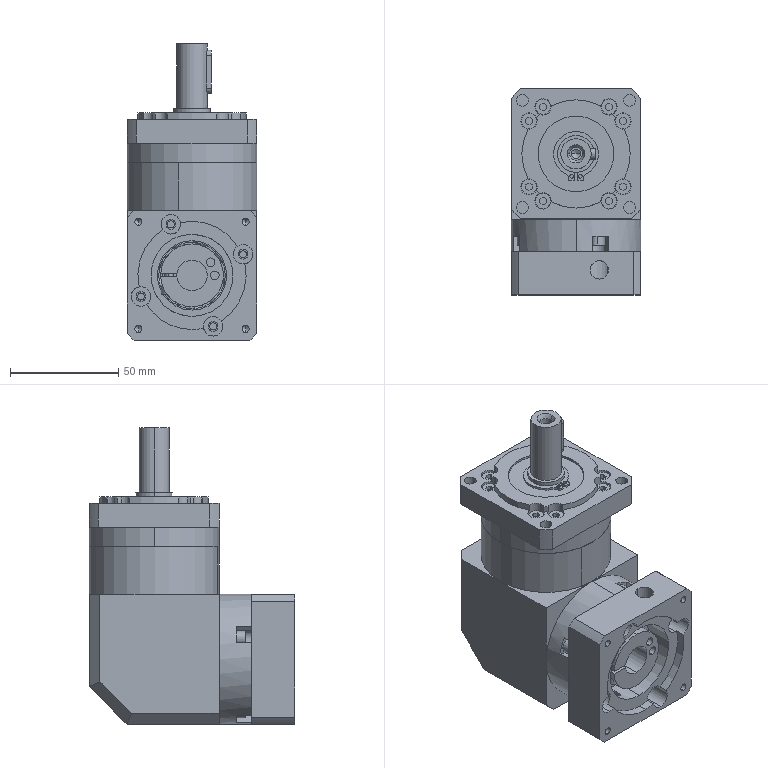Part | SolidWorks | features BaseBody 8 | 8 solids | 603 faces | box 60 x 95 x 137 mm | volume 414579 mm3 | plane 255 | cylinder 228 | spline 105 | cone 15 | commonest cylinder face diameters 7 x26 3.3 x18 7.5 x16 50 x14 20 x12 5 x10